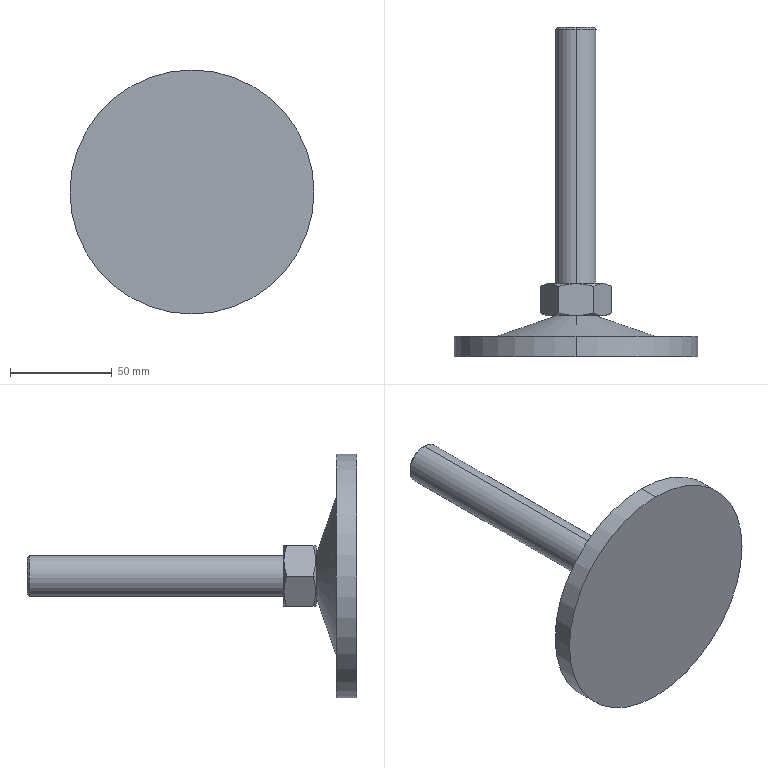Part | STEP file | Leveling Foot BF-20 | 2 solids | 83 faces | box 120 x 162 x 120 mm | volume 186987 mm3 | cone 48 | cylinder 24 | plane 11 | commonest cylinder face diameters 17.294 x20 20 x2 120 x2